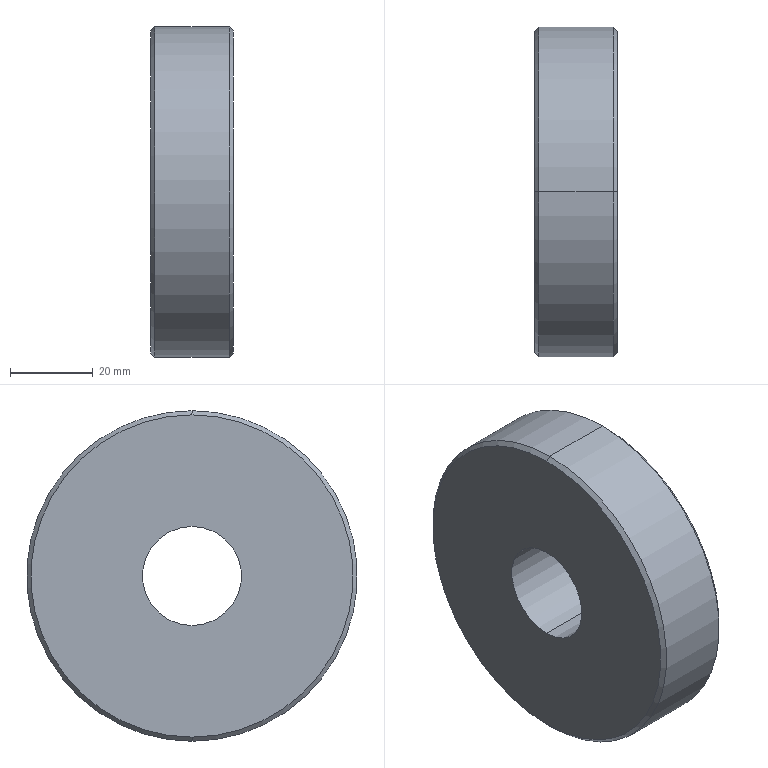Part | SolidWorks | features Chamfer 2, Cut 1, Extrusion 1 | 1 solid | 12 faces | box 20 x 80 x 80 mm | volume 90475 mm3 | cone 6 | cylinder 4 | plane 2 | commonest cylinder face diameters 24 x2 80 x2
STEP:
#1=CARTESIAN_POINT('',(16.825,0.,12.));
#2=VERTEX_POINT('',#1);
#3=CARTESIAN_POINT('',(16.825,0.,-12.));
#4=VERTEX_POINT('',#3);
#5=CARTESIAN_POINT('',(16.825,0.,0.));
#6=DIRECTION('',(1.,0.,0.));
#7=DIRECTION('',(0.,0.,-1.));
#8=AXIS2_PLACEMENT_3D('',#5,#6,#7);
#9=CIRCLE('',#8,12.);
#10=EDGE_CURVE('',#2,#4,#9,.T.);
#11=ORIENTED_EDGE('',*,*,#10,.F.);
#12=CARTESIAN_POINT('',(20.,0.,17.5));
#13=VERTEX_POINT('',#12);
#14=CARTESIAN_POINT('',(16.825,0.,12.));
#15=DIRECTION('',(0.5,0.,0.866));
#16=VECTOR('',#15,1000.);
#17=LINE('',#14,#16);
#18=EDGE_CURVE('',#2,#13,#17,.T.);
#19=ORIENTED_EDGE('',*,*,#18,.T.);
#20=CARTESIAN_POINT('',(20.,0.,-17.5));
#21=VERTEX_POINT('',#20);
#22=CARTESIAN_POINT('',(20.,0.,0.));
#23=DIRECTION('',(-1.,0.,0.));
#24=DIRECTION('',(0.,0.,-1.));
#25=AXIS2_PLACEMENT_3D('',#22,#23,#24);
#26=CIRCLE('',#25,17.5);
#27=EDGE_CURVE('',#21,#13,#26,.T.);
#28=ORIENTED_EDGE('',*,*,#27,.F.);
#29=CARTESIAN_POINT('',(16.825,0.,-12.));
#30=DIRECTION('',(0.5,0.,-0.866));
#31=VECTOR('',#30,1000.);
#32=LINE('',#29,#31);
#33=EDGE_CURVE('',#4,#21,#32,.T.);
#34=ORIENTED_EDGE('',*,*,#33,.F.);
#35=EDGE_LOOP('',(#11,#19,#28,#34));
#36=FACE_OUTER_BOUND('',#35,.T.);
#37=CARTESIAN_POINT('',(16.825,0.,0.));
#38=DIRECTION('',(1.,0.,0.));
#39=DIRECTION('',(0.,0.,-1.));
#40=AXIS2_PLACEMENT_3D('',#37,#38,#39);
#41=CONICAL_SURFACE('',#40,12.,1.047);
#42=ADVANCED_FACE('',(#36),#41,.F.);
#43=CARTESIAN_POINT('',(20.,0.,-39.));
#44=VERTEX_POINT('',#43);
#45=CARTESIAN_POINT('',(20.,0.,39.));
#46=VERTEX_POINT('',#45);
#47=CARTESIAN_POINT('',(20.,0.,0.));
#48=DIRECTION('',(1.,0.,0.));
#49=DIRECTION('',(0.,0.,-1.));
#50=AXIS2_PLACEMENT_3D('',#47,#48,#49);
#51=CIRCLE('',#50,39.);
#52=EDGE_CURVE('',#44,#46,#51,.T.);
#53=ORIENTED_EDGE('',*,*,#52,.F.);
#54=CARTESIAN_POINT('',(19.,0.,-40.));
#55=VERTEX_POINT('',#54);
#56=CARTESIAN_POINT('',(20.,0.,-39.));
#57=DIRECTION('',(-0.7071,0.,-0.7071));
#58=VECTOR('',#57,1000.);
#59=LINE('',#56,#58);
#60=EDGE_CURVE('',#44,#55,#59,.T.);
#61=ORIENTED_EDGE('',*,*,#60,.T.);
#62=CARTESIAN_POINT('',(19.,0.,40.));
#63=VERTEX_POINT('',#62);
#64=CARTESIAN_POINT('',(19.,0.,0.));
#65=DIRECTION('',(-1.,0.,0.));
#66=DIRECTION('',(0.,0.,-1.));
#67=AXIS2_PLACEMENT_3D('',#64,#65,#66);
#68=CIRCLE('',#67,40.);
#69=EDGE_CURVE('',#63,#55,#68,.T.);
#70=ORIENTED_EDGE('',*,*,#69,.F.);
#71=CARTESIAN_POINT('',(20.,0.,39.));
#72=DIRECTION('',(-0.7071,0.,0.7071));
#73=VECTOR('',#72,1000.);
#74=LINE('',#71,#73);
#75=EDGE_CURVE('',#46,#63,#74,.T.);
#76=ORIENTED_EDGE('',*,*,#75,.F.);
#77=EDGE_LOOP('',(#53,#61,#70,#76));
#78=FACE_OUTER_BOUND('',#77,.T.);
#79=CARTESIAN_POINT('',(20.,0.,0.));
#80=DIRECTION('',(-1.,0.,0.));
#81=DIRECTION('',(0.,0.,1.));
#82=AXIS2_PLACEMENT_3D('',#79,#80,#81);
#83=CONICAL_SURFACE('',#82,39.,0.7854);
#84=ADVANCED_FACE('',(#78),#83,.T.);
#85=CARTESIAN_POINT('',(0.,0.,39.));
#86=VERTEX_POINT('',#85);
#87=CARTESIAN_POINT('',(0.,0.,-39.));
#88=VERTEX_POINT('',#87);
#89=CARTESIAN_POINT('',(0.,0.,0.));
#90=DIRECTION('',(-1.,0.,0.));
#91=DIRECTION('',(0.,0.,-1.));
#92=AXIS2_PLACEMENT_3D('',#89,#90,#91);
#93=CIRCLE('',#92,39.);
#94=EDGE_CURVE('',#86,#88,#93,.T.);
#95=ORIENTED_EDGE('',*,*,#94,.F.);
#96=CARTESIAN_POINT('',(1.,0.,40.));
#97=VERTEX_POINT('',#96);
#98=CARTESIAN_POINT('',(1.,0.,40.));
#99=DIRECTION('',(0.7071,0.,0.7071));
#100=VECTOR('',#99,1000.);
#101=LINE('',#98,#100);
#102=EDGE_CURVE('',#86,#97,#101,.T.);
#103=ORIENTED_EDGE('',*,*,#102,.T.);
#104=CARTESIAN_POINT('',(1.,0.,-40.));
#105=VERTEX_POINT('',#104);
#106=CARTESIAN_POINT('',(1.,0.,0.));
#107=DIRECTION('',(1.,0.,0.));
#108=DIRECTION('',(0.,0.,-1.));
#109=AXIS2_PLACEMENT_3D('',#106,#107,#108);
#110=CIRCLE('',#109,40.);
#111=EDGE_CURVE('',#105,#97,#110,.T.);
#112=ORIENTED_EDGE('',*,*,#111,.F.);
#113=CARTESIAN_POINT('',(1.,0.,-40.));
#114=DIRECTION('',(0.7071,0.,-0.7071));
#115=VECTOR('',#114,1000.);
#116=LINE('',#113,#115);
#117=EDGE_CURVE('',#88,#105,#116,.T.);
#118=ORIENTED_EDGE('',*,*,#117,.F.);
#119=EDGE_LOOP('',(#95,#103,#112,#118));
#120=FACE_OUTER_BOUND('',#119,.T.);
#121=CARTESIAN_POINT('',(1.,0.,0.));
#122=DIRECTION('',(1.,0.,0.));
#123=DIRECTION('',(0.,0.,-1.));
#124=AXIS2_PLACEMENT_3D('',#121,#122,#123);
#125=CONICAL_SURFACE('',#124,40.,0.7854);
#126=ADVANCED_FACE('',(#120),#125,.T.);
#127=CARTESIAN_POINT('',(0.,0.,12.));
#128=VERTEX_POINT('',#127);
#129=CARTESIAN_POINT('',(0.,0.,-12.));
#130=VERTEX_POINT('',#129);
#131=CARTESIAN_POINT('',(0.,0.,0.));
#132=DIRECTION('',(1.,0.,0.));
#133=DIRECTION('',(0.,0.,-1.));
#134=AXIS2_PLACEMENT_3D('',#131,#132,#133);
#135=CIRCLE('',#134,12.);
#136=EDGE_CURVE('',#128,#130,#135,.T.);
#137=ORIENTED_EDGE('',*,*,#136,.F.);
#138=CARTESIAN_POINT('',(0.,0.,12.));
#139=DIRECTION('',(1.,0.,0.));
#140=VECTOR('',#139,1000.);
#141=LINE('',#138,#140);
#142=EDGE_CURVE('',#128,#2,#141,.T.);
#143=ORIENTED_EDGE('',*,*,#142,.T.);
#144=ORIENTED_EDGE('',*,*,#10,.T.);
#145=CARTESIAN_POINT('',(0.,0.,-12.));
#146=DIRECTION('',(1.,0.,0.));
#147=VECTOR('',#146,1000.);
#148=LINE('',#145,#147);
#149=EDGE_CURVE('',#130,#4,#148,.T.);
#150=ORIENTED_EDGE('',*,*,#149,.F.);
#151=EDGE_LOOP('',(#137,#143,#144,#150));
#152=FACE_OUTER_BOUND('',#151,.T.);
#153=CARTESIAN_POINT('',(0.,0.,0.));
#154=DIRECTION('',(1.,0.,0.));
#155=DIRECTION('',(0.,0.,-1.));
#156=AXIS2_PLACEMENT_3D('',#153,#154,#155);
#157=CYLINDRICAL_SURFACE('',#156,12.);
#158=ADVANCED_FACE('',(#152),#157,.F.);
#159=ORIENTED_EDGE('',*,*,#69,.T.);
#160=CARTESIAN_POINT('',(20.,0.,-40.));
#161=DIRECTION('',(-1.,0.,0.));
#162=VECTOR('',#161,1000.);
#163=LINE('',#160,#162);
#164=EDGE_CURVE('',#55,#105,#163,.T.);
#165=ORIENTED_EDGE('',*,*,#164,.T.);
#166=ORIENTED_EDGE('',*,*,#111,.T.);
#167=CARTESIAN_POINT('',(20.,0.,40.));
#168=DIRECTION('',(-1.,0.,0.));
#169=VECTOR('',#168,1000.);
#170=LINE('',#167,#169);
#171=EDGE_CURVE('',#63,#97,#170,.T.);
#172=ORIENTED_EDGE('',*,*,#171,.F.);
#173=EDGE_LOOP('',(#159,#165,#166,#172));
#174=FACE_OUTER_BOUND('',#173,.T.);
#175=CARTESIAN_POINT('',(20.,0.,0.));
#176=DIRECTION('',(-1.,0.,0.));
#177=DIRECTION('',(0.,0.,1.));
#178=AXIS2_PLACEMENT_3D('',#175,#176,#177);
#179=CYLINDRICAL_SURFACE('',#178,40.);
#180=ADVANCED_FACE('',(#174),#179,.T.);
#181=ORIENTED_EDGE('',*,*,#164,.F.);
#182=CARTESIAN_POINT('',(19.,0.,0.));
#183=DIRECTION('',(-1.,0.,0.));
#184=DIRECTION('',(0.,0.,-1.));
#185=AXIS2_PLACEMENT_3D('',#182,#183,#184);
#186=CIRCLE('',#185,40.);
#187=EDGE_CURVE('',#55,#63,#186,.T.);
#188=ORIENTED_EDGE('',*,*,#187,.T.);
#189=ORIENTED_EDGE('',*,*,#171,.T.);
#190=CARTESIAN_POINT('',(1.,0.,0.));
#191=DIRECTION('',(1.,0.,0.));
#192=DIRECTION('',(0.,0.,-1.));
#193=AXIS2_PLACEMENT_3D('',#190,#191,#192);
#194=CIRCLE('',#193,40.);
#195=EDGE_CURVE('',#97,#105,#194,.T.);
#196=ORIENTED_EDGE('',*,*,#195,.T.);
#197=EDGE_LOOP('',(#181,#188,#189,#196));
#198=FACE_OUTER_BOUND('',#197,.T.);
#199=CARTESIAN_POINT('',(20.,0.,0.));
#200=DIRECTION('',(-1.,0.,0.));
#201=DIRECTION('',(0.,0.,1.));
#202=AXIS2_PLACEMENT_3D('',#199,#200,#201);
#203=CYLINDRICAL_SURFACE('',#202,40.);
#204=ADVANCED_FACE('',(#198),#203,.T.);
#205=ORIENTED_EDGE('',*,*,#27,.T.);
#206=CARTESIAN_POINT('',(20.,0.,0.));
#207=DIRECTION('',(-1.,0.,0.));
#208=DIRECTION('',(0.,0.,-1.));
#209=AXIS2_PLACEMENT_3D('',#206,#207,#208);
#210=CIRCLE('',#209,17.5);
#211=EDGE_CURVE('',#13,#21,#210,.T.);
#212=ORIENTED_EDGE('',*,*,#211,.T.);
#213=EDGE_LOOP('',(#205,#212));
#214=FACE_BOUND('',#213,.T.);
#215=CARTESIAN_POINT('',(20.,0.,0.));
#216=DIRECTION('',(1.,0.,0.));
#217=DIRECTION('',(0.,0.,-1.));
#218=AXIS2_PLACEMENT_3D('',#215,#216,#217);
#219=CIRCLE('',#218,39.);
#220=EDGE_CURVE('',#46,#44,#219,.T.);
#221=ORIENTED_EDGE('',*,*,#220,.T.);
#222=ORIENTED_EDGE('',*,*,#52,.T.);
#223=EDGE_LOOP('',(#221,#222));
#224=FACE_OUTER_BOUND('',#223,.T.);
#225=CARTESIAN_POINT('',(20.,0.,0.));
#226=DIRECTION('',(1.,0.,0.));
#227=DIRECTION('',(0.,0.,-1.));
#228=AXIS2_PLACEMENT_3D('',#225,#226,#227);
#229=PLANE('',#228);
#230=ADVANCED_FACE('',(#214,#224),#229,.T.);
#231=CARTESIAN_POINT('',(0.,0.,0.));
#232=DIRECTION('',(-1.,0.,0.));
#233=DIRECTION('',(0.,0.,-1.));
#234=AXIS2_PLACEMENT_3D('',#231,#232,#233);
#235=CIRCLE('',#234,39.);
#236=EDGE_CURVE('',#88,#86,#235,.T.);
#237=ORIENTED_EDGE('',*,*,#236,.T.);
#238=ORIENTED_EDGE('',*,*,#94,.T.);
#239=EDGE_LOOP('',(#237,#238));
#240=FACE_OUTER_BOUND('',#239,.T.);
#241=CARTESIAN_POINT('',(0.,0.,0.));
#242=DIRECTION('',(1.,0.,0.));
#243=DIRECTION('',(0.,0.,-1.));
#244=AXIS2_PLACEMENT_3D('',#241,#242,#243);
#245=CIRCLE('',#244,12.);
#246=EDGE_CURVE('',#130,#128,#245,.T.);
#247=ORIENTED_EDGE('',*,*,#246,.T.);
#248=ORIENTED_EDGE('',*,*,#136,.T.);
#249=EDGE_LOOP('',(#247,#248));
#250=FACE_BOUND('',#249,.T.);
#251=CARTESIAN_POINT('',(0.,0.,0.));
#252=DIRECTION('',(1.,0.,0.));
#253=DIRECTION('',(0.,0.,-1.));
#254=AXIS2_PLACEMENT_3D('',#251,#252,#253);
#255=PLANE('',#254);
#256=ADVANCED_FACE('',(#240,#250),#255,.F.);
#257=ORIENTED_EDGE('',*,*,#142,.F.);
#258=ORIENTED_EDGE('',*,*,#246,.F.);
#259=ORIENTED_EDGE('',*,*,#149,.T.);
#260=CARTESIAN_POINT('',(16.825,0.,0.));
#261=DIRECTION('',(1.,0.,0.));
#262=DIRECTION('',(0.,0.,-1.));
#263=AXIS2_PLACEMENT_3D('',#260,#261,#262);
#264=CIRCLE('',#263,12.);
#265=EDGE_CURVE('',#4,#2,#264,.T.);
#266=ORIENTED_EDGE('',*,*,#265,.T.);
#267=EDGE_LOOP('',(#257,#258,#259,#266));
#268=FACE_OUTER_BOUND('',#267,.T.);
#269=CARTESIAN_POINT('',(0.,0.,0.));
#270=DIRECTION('',(1.,0.,0.));
#271=DIRECTION('',(0.,0.,-1.));
#272=AXIS2_PLACEMENT_3D('',#269,#270,#271);
#273=CYLINDRICAL_SURFACE('',#272,12.);
#274=ADVANCED_FACE('',(#268),#273,.F.);
#275=ORIENTED_EDGE('',*,*,#102,.F.);
#276=ORIENTED_EDGE('',*,*,#236,.F.);
#277=ORIENTED_EDGE('',*,*,#117,.T.);
#278=ORIENTED_EDGE('',*,*,#195,.F.);
#279=EDGE_LOOP('',(#275,#276,#277,#278));
#280=FACE_OUTER_BOUND('',#279,.T.);
#281=CARTESIAN_POINT('',(1.,0.,0.));
#282=DIRECTION('',(1.,0.,0.));
#283=DIRECTION('',(0.,0.,-1.));
#284=AXIS2_PLACEMENT_3D('',#281,#282,#283);
#285=CONICAL_SURFACE('',#284,40.,0.7854);
#286=ADVANCED_FACE('',(#280),#285,.T.);
#287=ORIENTED_EDGE('',*,*,#60,.F.);
#288=ORIENTED_EDGE('',*,*,#220,.F.);
#289=ORIENTED_EDGE('',*,*,#75,.T.);
#290=ORIENTED_EDGE('',*,*,#187,.F.);
#291=EDGE_LOOP('',(#287,#288,#289,#290));
#292=FACE_OUTER_BOUND('',#291,.T.);
#293=CARTESIAN_POINT('',(20.,0.,0.));
#294=DIRECTION('',(-1.,0.,0.));
#295=DIRECTION('',(0.,0.,1.));
#296=AXIS2_PLACEMENT_3D('',#293,#294,#295);
#297=CONICAL_SURFACE('',#296,39.,0.7854);
#298=ADVANCED_FACE('',(#292),#297,.T.);
#299=ORIENTED_EDGE('',*,*,#18,.F.);
#300=ORIENTED_EDGE('',*,*,#265,.F.);
#301=ORIENTED_EDGE('',*,*,#33,.T.);
#302=ORIENTED_EDGE('',*,*,#211,.F.);
#303=EDGE_LOOP('',(#299,#300,#301,#302));
#304=FACE_OUTER_BOUND('',#303,.T.);
#305=CARTESIAN_POINT('',(16.825,0.,0.));
#306=DIRECTION('',(1.,0.,0.));
#307=DIRECTION('',(0.,0.,-1.));
#308=AXIS2_PLACEMENT_3D('',#305,#306,#307);
#309=CONICAL_SURFACE('',#308,12.,1.047);
#310=ADVANCED_FACE('',(#304),#309,.F.);
#311=CLOSED_SHELL('',(#42,#84,#126,#158,#180,#204,#230,#256,#274,#286,#298,#310));
#312=MANIFOLD_SOLID_BREP('',#311);
#313=CARTESIAN_POINT('',(0.,0.,0.));
#314=DIRECTION('',(0.,0.,1.));
#315=DIRECTION('',(1.,0.,0.));
#316=AXIS2_PLACEMENT_3D('',#313,#314,#315);
#317=(LENGTH_UNIT()NAMED_UNIT(*)SI_UNIT(.MILLI.,.METRE.));
#318=UNCERTAINTY_MEASURE_WITH_UNIT(LENGTH_MEASURE(0.00001),#317,'','');
#319=(NAMED_UNIT(*)PLANE_ANGLE_UNIT()SI_UNIT($,.RADIAN.));
#320=(NAMED_UNIT(*)SI_UNIT($,.STERADIAN.)SOLID_ANGLE_UNIT());
#321=(GEOMETRIC_REPRESENTATION_CONTEXT(3)GLOBAL_UNCERTAINTY_ASSIGNED_CONTEXT((#318))GLOBAL_UNIT_ASSIGNED_CONTEXT((#317,#319,#320))REPRESENTATION_CONTEXT('',''));
#322=ADVANCED_BREP_SHAPE_REPRESENTATION('',(#312,#316),#321);